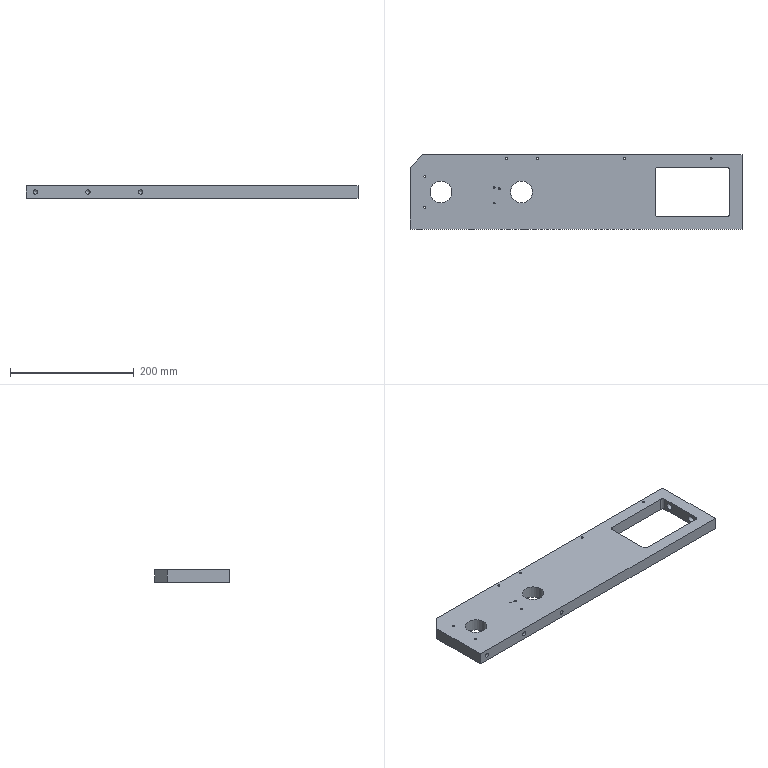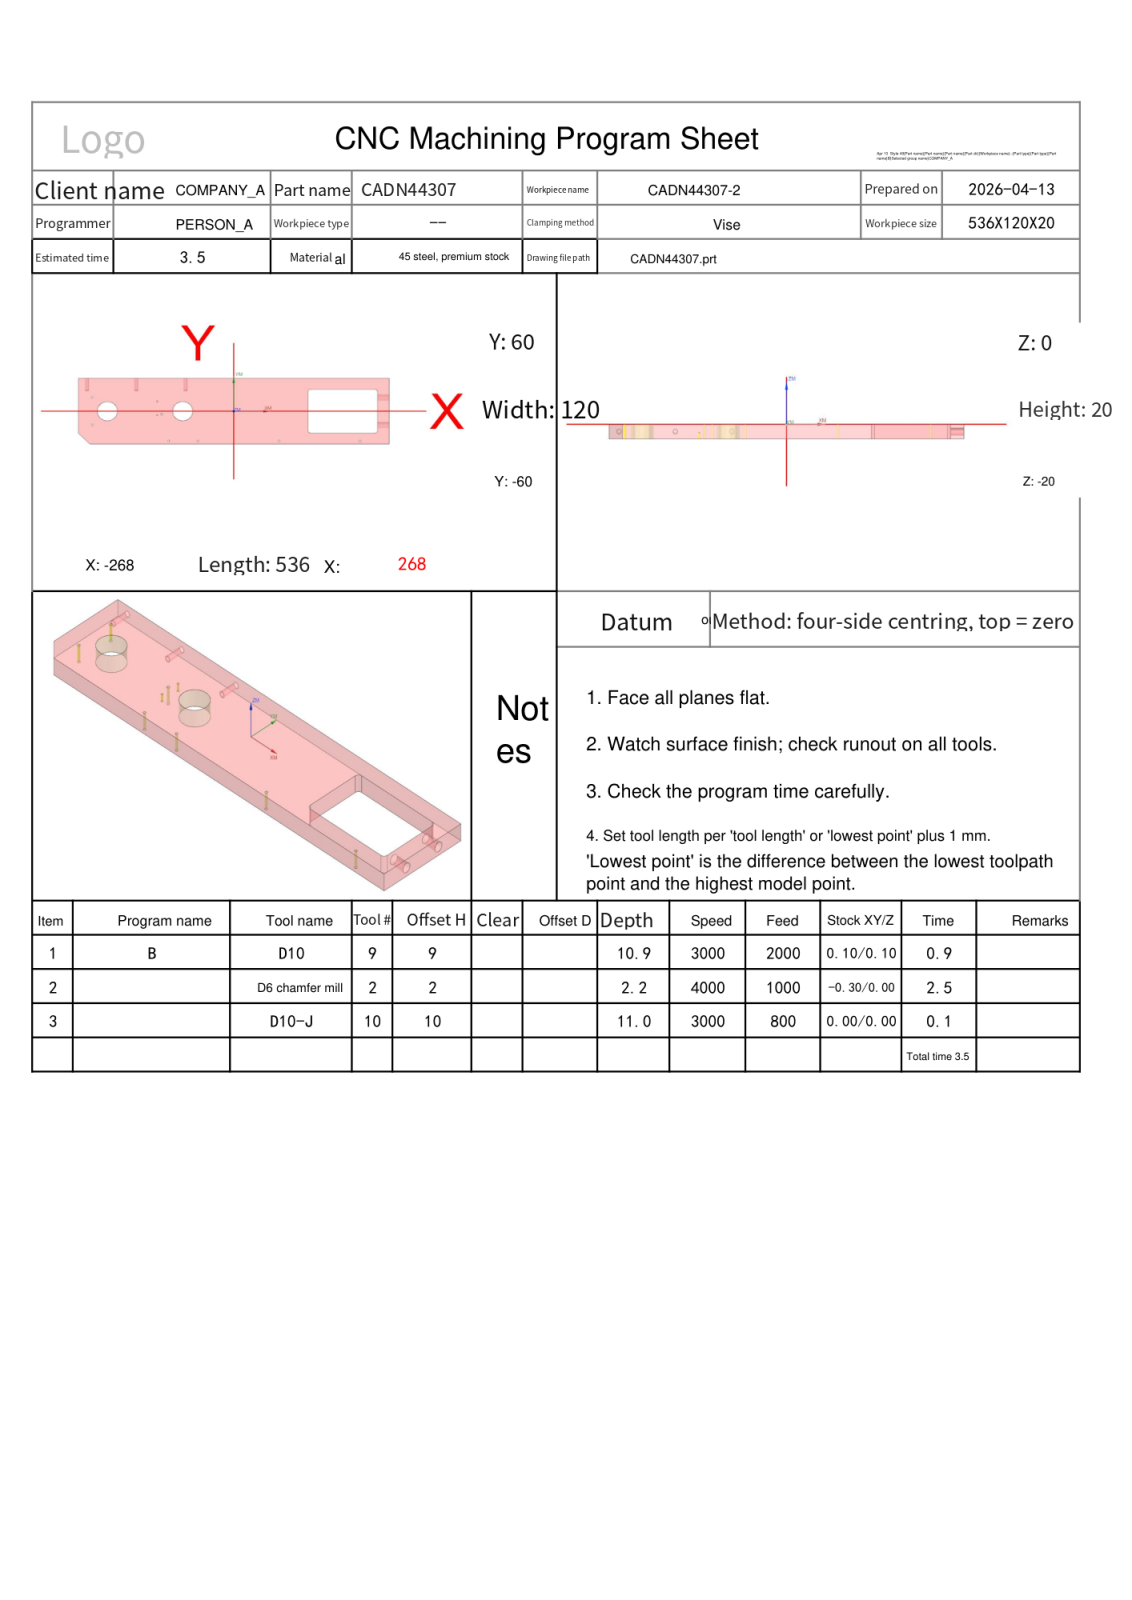NC program | NX | posted by the shop | part box 536 x 120 x 20 mm
Whole program:
%
O0001
(Machine time: 3.97 MIN)
(===Total Tool:3===)
(T9=D10     D=10.  R=0.   D-  H09 Z=-10.9 )
(T2=D6 chamfer mill   D=6.   R=0.   D-  H02 Z=-2.2  )
(T10=D10-J  D=10.  R=0.   D-  H10 Z=-11.  )
G80 G90 G17 G49 G40
G91 G28 Z0
M01
N1 T09 M06
(D10  D=10. R=0. H=09 ce=0.10 di=0.10)
G00 G90 G54 X-245.242 Y-69.97 M03 S3000
G43 H09 Z20.
M08
Z-.3
G01 X-251.606 Y-63.606 F2000.
X-271.606 Y-43.606
X-277.97 Y-37.242
G00 Z-.6
G01 X-271.606 Y-43.606
X-251.606 Y-63.606
X-245.242 Y-69.97
G00 Z-.9
G01 X-251.606 Y-63.606
X-271.606 Y-43.606
X-277.97 Y-37.242
G00 Z-1.2
G01 X-271.606 Y-43.606
X-251.606 Y-63.606
X-245.242 Y-69.97
G00 Z-1.5
G01 X-251.606 Y-63.606
X-271.606 Y-43.606
X-277.97 Y-37.242
G00 Z-1.8
G01 X-271.606 Y-43.606
X-251.606 Y-63.606
X-245.242 Y-69.97
G00 Z-2.1
G01 X-251.606 Y-63.606
X-271.606 Y-43.606
X-277.97 Y-37.242
G00 Z-2.4
G01 X-271.606 Y-43.606
X-251.606 Y-63.606
X-245.242 Y-69.97
G00 Z-2.7
G01 X-251.606 Y-63.606
X-271.606 Y-43.606
X-277.97 Y-37.242
G00 Z-3.
G01 X-271.606 Y-43.606
X-251.606 Y-63.606
X-245.242 Y-69.97
G00 Z-3.3
G01 X-251.606 Y-63.606
X-271.606 Y-43.606
X-277.97 Y-37.242
G00 Z-3.6
G01 X-271.606 Y-43.606
X-251.606 Y-63.606
X-245.242 Y-69.97
G00 Z-3.9
G01 X-251.606 Y-63.606
X-271.606 Y-43.606
X-277.97 Y-37.242
G00 Z-4.2
G01 X-271.606 Y-43.606
X-251.606 Y-63.606
X-245.242 Y-69.97
G00 Z-4.5
G01 X-251.606 Y-63.606
X-271.606 Y-43.606
X-277.97 Y-37.242
G00 Z-4.8
G01 X-271.606 Y-43.606
X-251.606 Y-63.606
X-245.242 Y-69.97
G00 Z-5.1
G01 X-251.606 Y-63.606
X-271.606 Y-43.606
X-277.97 Y-37.242
G00 Z-5.4
G01 X-271.606 Y-43.606
X-251.606 Y-63.606
X-245.242 Y-69.97
G00 Z-5.7
G01 X-251.606 Y-63.606
X-271.606 Y-43.606
X-277.97 Y-37.242
G00 Z-6.
G01 X-271.606 Y-43.606
X-251.606 Y-63.606
X-245.242 Y-69.97
G00 Z-6.3
G01 X-251.606 Y-63.606
X-271.606 Y-43.606
X-277.97 Y-37.242
G00 Z-6.6
G01 X-271.606 Y-43.606
X-251.606 Y-63.606
X-245.242 Y-69.97
G00 Z-6.9
G01 X-251.606 Y-63.606
X-271.606 Y-43.606
X-277.97 Y-37.242
G00 Z-7.2
G01 X-271.606 Y-43.606
X-251.606 Y-63.606
X-245.242 Y-69.97
G00 Z-7.5
G01 X-251.606 Y-63.606
X-271.606 Y-43.606
X-277.97 Y-37.242
G00 Z-7.8
G01 X-271.606 Y-43.606
X-251.606 Y-63.606
X-245.242 Y-69.97
G00 Z-8.1
G01 X-251.606 Y-63.606
X-271.606 Y-43.606
X-277.97 Y-37.242
G00 Z-8.4
G01 X-271.606 Y-43.606
X-251.606 Y-63.606
X-245.242 Y-69.97
G00 Z-8.7
G01 X-251.606 Y-63.606
X-271.606 Y-43.606
X-277.97 Y-37.242
G00 Z-9.
G01 X-271.606 Y-43.606
X-251.606 Y-63.606
X-245.242 Y-69.97
G00 Z-9.3
G01 X-251.606 Y-63.606
X-271.606 Y-43.606
X-277.97 Y-37.242
G00 Z-9.6
G01 X-271.606 Y-43.606
X-251.606 Y-63.606
X-245.242 Y-69.97
G00 Z-9.9
G01 X-251.606 Y-63.606
X-271.606 Y-43.606
X-277.97 Y-37.242
G00 Z-10.2
G01 X-271.606 Y-43.606
X-251.606 Y-63.606
X-245.242 Y-69.97
G00 Z-10.5
G01 X-251.606 Y-63.606
X-271.606 Y-43.606
X-277.97 Y-37.242
G00 Z-10.8
G01 X-271.606 Y-43.606
X-251.606 Y-63.606
X-245.242 Y-69.97
G00 Z-10.9
G01 X-251.606 Y-63.606
X-271.606 Y-43.606
X-277.97 Y-37.242
G00 Z20.
G91 G28 Z0.0
M05
M09
G91 G28 Z0.0
M01
N2 T02 M06
(D6 chamfer mill  D=6. R=0. H=02 ce=0.00 di=0.10)
G00 G90 G54 X-244. Y-25. M03 S2000
G43 H02 Z20.
M08
G98 G81 X-244. Y-25. Z-2.2 R3. F100.
Y25.
X-124. Y-5.25
X-112. Y-54.25
X-62.
X78.
X218.
G80
G00 Z20.
G00 G90 X136.724 Y39.1 M03 S4000
Z20.
Z2.5
G01 X132.843 Z1.088 F1000.
X132.407 Y39.06 Z.928
X131.978 Y38.974 Z.769
X131.561 Y38.842 Z.61
X131.159 Y38.667 Z.45
X130.779 Y38.45 Z.291
X130.424 Y38.194 Z.132
X130.099 Y37.901 Z-.028
X129.806 Y37.576 Z-.187
X129.55 Y37.221 Z-.346
X129.333 Y36.841 Z-.506
X129.158 Y36.439 Z-.665
X129.026 Y36.022 Z-.824
X128.94 Y35.593 Z-.984
X128.9 Y35.157 Z-1.143
Y35. Z-1.2
Y-35.
G03 X133. Y-39.1 I4.1 J0.0
G01 X243.
G03 X247.1 Y-35. I0.0 J4.1
G01 Y35.
G03 X243. Y39.1 I-4.1 J0.0
G01 X133.
G03 X128.9 Y35. I0.0 J-4.1
G01 Y34.5
Z1.3
G00 Z20.
X-268.9 Y51.422
Z2.5
G01 Y59.785 Z-.544
X-268.866 Y59.997 Z-.622
X-268.794 Y60.199 Z-.7
X-268.688 Y60.386 Z-.778
X-268.551 Y60.551 Z-.857
X-268.386 Y60.688 Z-.935
X-268.199 Y60.794 Z-1.013
X-267.997 Y60.866 Z-1.091
X-267.785 Y60.9 Z-1.169
X-267.7 Z-1.2
X267.7
G02 X268.9 Y59.7 I0.0 J-1.2
G01 Y-59.7
G02 X267.7 Y-60.9 I-1.2 J0.0
G01 X-247.876
G02 X-248.724 Y-60.549 I0.0 J1.2
G01 X-268.549 Y-40.724
G02 X-268.9 Y-39.876 I.849 J.849
G01 Y59.7
G02 X-267.7 Y60.9 I1.2 J0.0
G01 X-267.2
Z1.3
G00 Z20.
X-74.417 Y-9.541
Z2.5
G01 X-74.288 Y-9.361 Z2.419
X-73.813 Y-8.626 Z2.101
X-73.379 Y-7.866 Z1.782
X-72.984 Y-7.084 Z1.464
X-72.632 Y-6.283 Z1.145
X-72.322 Y-5.464 Z.826
X-72.056 Y-4.631 Z.508
X-71.834 Y-3.784 Z.189
X-71.657 Y-2.927 Z-.129
X-71.525 Y-2.061 Z-.448
X-71.44 Y-1.19 Z-.767
X-71.4 Y-.316 Z-1.085
Y0.0 Z-1.2
G03 X-88. Y16.6 I-16.6 J0.0
X-104.6 Y0.0 I0.0 J-16.6
X-88. Y-16.6 I16.6 J0.0
X-71.4 Y0.0 I0.0 J16.6
X-71.408 Y.5 I-16.6 J0.0
G01 Z1.3
G00 Z20.
X-204.417 Y-9.541
Z2.5
G01 X-204.288 Y-9.361 Z2.419
X-203.813 Y-8.626 Z2.101
X-203.379 Y-7.866 Z1.782
X-202.984 Y-7.084 Z1.464
X-202.632 Y-6.283 Z1.145
X-202.322 Y-5.464 Z.826
X-202.056 Y-4.631 Z.508
X-201.834 Y-3.784 Z.189
X-201.657 Y-2.927 Z-.129
X-201.525 Y-2.061 Z-.448
X-201.44 Y-1.19 Z-.767
X-201.4 Y-.316 Z-1.085
Y0.0 Z-1.2
G03 X-218. Y16.6 I-16.6 J0.0
X-234.6 Y0.0 I0.0 J-16.6
X-218. Y-16.6 I16.6 J0.0
X-201.4 Y0.0 I0.0 J16.6
X-201.408 Y.5 I-16.6 J0.0
G01 Z1.3
G00 Z20.
G91 G28 Z0.0
M05
M09
G91 G28 Z0.0
M01
N3 T10 M06
(D10-J  D=10. R=0. H=10 ce=0.00 di=0.00)
G00 G90 G54 X-247.293 Y-67.778 M03 S3000
G43 H10 Z20.
M08
Z-10.
G01 Z-11. F800.
X-251.536 Y-63.536
X-271.536 Y-43.536
X-275.778 Y-39.293
Z-10.
G00 Z20.
M05
M09
G91 G28 Z0.0
G91 G28 Y0.0
M30
%